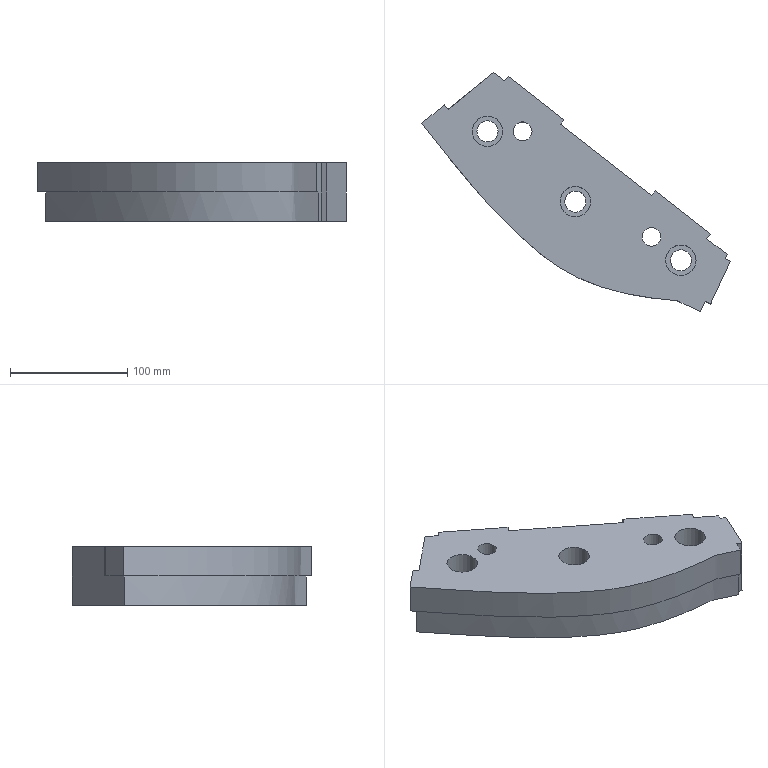Part | NX | features solid 2 | 1 solid | 34 faces | box 263.418 x 204.229 x 50 mm | volume 1065155 mm3 | plane 23 | cylinder 8 | spline 3 | commonest cylinder face diameters 18 x3 26 x3 16 x2
STEP:
#1=CARTESIAN_POINT('',(148.001,-494.484,-50.));
#2=VERTEX_POINT('',#1);
#3=CARTESIAN_POINT('',(140.001,-494.484,-50.));
#4=DIRECTION('',(0.,0.,1.));
#5=DIRECTION('',(1.,0.,0.));
#6=AXIS2_PLACEMENT_3D('',#3,#4,#5);
#7=CIRCLE('',#6,8.);
#8=EDGE_CURVE('',#2,#2,#7,.F.);
#9=ORIENTED_EDGE('',*,*,#8,.F.);
#10=EDGE_LOOP('',(#9));
#11=FACE_BOUND('',#10,.T.);
#12=CARTESIAN_POINT('',(38.001,-404.484,-50.));
#13=VERTEX_POINT('',#12);
#14=CARTESIAN_POINT('',(30.001,-404.484,-50.));
#15=DIRECTION('',(0.,0.,1.));
#16=DIRECTION('',(1.,0.,0.));
#17=AXIS2_PLACEMENT_3D('',#14,#15,#16);
#18=CIRCLE('',#17,8.);
#19=EDGE_CURVE('',#13,#13,#18,.F.);
#20=ORIENTED_EDGE('',*,*,#19,.F.);
#21=EDGE_LOOP('',(#20));
#22=FACE_BOUND('',#21,.T.);
#23=CARTESIAN_POINT('',(183.872,-553.837,-50.));
#24=VERTEX_POINT('',#23);
#25=CARTESIAN_POINT('',(-49.164,-398.414,-50.));
#26=VERTEX_POINT('',#25);
#27=CARTESIAN_POINT('',(183.872,-553.837,-50.));
#28=CARTESIAN_POINT('',(181.19,-552.587,-50.));
#29=CARTESIAN_POINT('',(177.655,-550.938,-50.));
#30=CARTESIAN_POINT('',(173.916,-549.195,-50.));
#31=CARTESIAN_POINT('',(171.6,-548.115,-50.));
#32=CARTESIAN_POINT('',(169.771,-547.262,-50.));
#33=CARTESIAN_POINT('',(168.654,-546.741,-50.));
#34=CARTESIAN_POINT('',(168.003,-546.437,-50.));
#35=CARTESIAN_POINT('',(167.64,-546.268,-50.));
#36=CARTESIAN_POINT('',(167.426,-546.168,-50.));
#37=CARTESIAN_POINT('',(167.355,-546.135,-50.));
#38=CARTESIAN_POINT('',(167.291,-546.104,-50.));
#39=CARTESIAN_POINT('',(167.361,-546.137,-50.));
#40=CARTESIAN_POINT('',(167.014,-545.975,-50.));
#41=CARTESIAN_POINT('',(166.698,-545.827,-50.));
#42=CARTESIAN_POINT('',(166.252,-545.617,-50.));
#43=CARTESIAN_POINT('',(165.74,-545.378,-50.));
#44=CARTESIAN_POINT('',(165.042,-545.046,-50.));
#45=CARTESIAN_POINT('',(164.226,-544.695,-50.));
#46=CARTESIAN_POINT('',(163.094,-544.305,-50.));
#47=CARTESIAN_POINT('',(162.195,-544.064,-50.));
#48=CARTESIAN_POINT('',(161.539,-543.93,-50.));
#49=CARTESIAN_POINT('',(161.184,-543.867,-50.));
#50=CARTESIAN_POINT('',(160.858,-543.817,-50.));
#51=CARTESIAN_POINT('',(160.755,-543.804,-50.));
#52=CARTESIAN_POINT('',(160.477,-543.771,-50.));
#53=CARTESIAN_POINT('',(160.073,-543.731,-50.));
#54=CARTESIAN_POINT('',(159.523,-543.683,-50.));
#55=CARTESIAN_POINT('',(159.037,-543.643,-50.));
#56=CARTESIAN_POINT('',(158.567,-543.607,-50.));
#57=CARTESIAN_POINT('',(158.321,-543.588,-50.));
#58=CARTESIAN_POINT('',(157.916,-543.557,-50.));
#59=CARTESIAN_POINT('',(157.244,-543.504,-50.));
#60=CARTESIAN_POINT('',(156.27,-543.425,-50.));
#61=CARTESIAN_POINT('',(155.116,-543.328,-50.));
#62=CARTESIAN_POINT('',(153.584,-543.194,-50.));
#63=CARTESIAN_POINT('',(151.666,-543.017,-50.));
#64=CARTESIAN_POINT('',(149.486,-542.802,-50.));
#65=CARTESIAN_POINT('',(146.978,-542.536,-50.));
#66=CARTESIAN_POINT('',(143.79,-542.173,-50.));
#67=CARTESIAN_POINT('',(138.237,-541.478,-50.));
#68=CARTESIAN_POINT('',(130.582,-540.33,-50.));
#69=CARTESIAN_POINT('',(123.224,-538.968,-50.));
#70=CARTESIAN_POINT('',(118.275,-537.912,-50.));
#71=CARTESIAN_POINT('',(115.449,-537.265,-50.));
#72=CARTESIAN_POINT('',(113.484,-536.797,-50.));
#73=CARTESIAN_POINT('',(111.045,-536.188,-50.));
#74=CARTESIAN_POINT('',(108.002,-535.388,-50.));
#75=CARTESIAN_POINT('',(102.684,-533.89,-50.));
#76=CARTESIAN_POINT('',(95.378,-531.535,-50.));
#77=CARTESIAN_POINT('',(88.413,-528.888,-50.));
#78=CARTESIAN_POINT('',(83.006,-526.572,-50.));
#79=CARTESIAN_POINT('',(79.163,-524.8,-50.));
#80=CARTESIAN_POINT('',(75.001,-522.73,-50.));
#81=CARTESIAN_POINT('',(71.042,-520.6,-50.));
#82=CARTESIAN_POINT('',(67.801,-518.726,-50.));
#83=CARTESIAN_POINT('',(65.566,-517.361,-50.));
#84=CARTESIAN_POINT('',(64.317,-516.578,-50.));
#85=CARTESIAN_POINT('',(63.338,-515.952,-50.));
#86=CARTESIAN_POINT('',(62.553,-515.443,-50.));
#87=CARTESIAN_POINT('',(61.419,-514.694,-50.));
#88=CARTESIAN_POINT('',(59.423,-513.345,-50.));
#89=CARTESIAN_POINT('',(56.429,-511.236,-50.));
#90=CARTESIAN_POINT('',(53.281,-508.908,-50.));
#91=CARTESIAN_POINT('',(50.978,-507.148,-50.));
#92=CARTESIAN_POINT('',(49.656,-506.124,-50.));
#93=CARTESIAN_POINT('',(48.597,-505.295,-50.));
#94=CARTESIAN_POINT('',(47.737,-504.616,-50.));
#95=CARTESIAN_POINT('',(46.527,-503.654,-50.));
#96=CARTESIAN_POINT('',(44.454,-501.988,-50.));
#97=CARTESIAN_POINT('',(41.508,-499.566,-50.));
#98=CARTESIAN_POINT('',(38.048,-496.635,-50.));
#99=CARTESIAN_POINT('',(34.6,-493.624,-50.));
#100=CARTESIAN_POINT('',(31.367,-490.714,-50.));
#101=CARTESIAN_POINT('',(28.058,-487.655,-50.));
#102=CARTESIAN_POINT('',(25.286,-485.02,-50.));
#103=CARTESIAN_POINT('',(23.09,-482.892,-50.));
#104=CARTESIAN_POINT('',(21.348,-481.181,-50.));
#105=CARTESIAN_POINT('',(19.949,-479.79,-50.));
#106=CARTESIAN_POINT('',(17.948,-477.781,-50.));
#107=CARTESIAN_POINT('',(14.47,-474.232,-50.));
#108=CARTESIAN_POINT('',(10.396,-469.946,-50.));
#109=CARTESIAN_POINT('',(6.255,-465.465,-50.));
#110=CARTESIAN_POINT('',(3.108,-461.998,-50.));
#111=CARTESIAN_POINT('',(0.4635,-459.035,-50.));
#112=CARTESIAN_POINT('',(-1.422,-456.894,-50.));
#113=CARTESIAN_POINT('',(-2.477,-455.691,-50.));
#114=CARTESIAN_POINT('',(-3.348,-454.691,-50.));
#115=CARTESIAN_POINT('',(-3.921,-454.032,-50.));
#116=CARTESIAN_POINT('',(-4.799,-453.019,-50.));
#117=CARTESIAN_POINT('',(-6.306,-451.271,-50.));
#118=CARTESIAN_POINT('',(-8.542,-448.656,-50.));
#119=CARTESIAN_POINT('',(-11.305,-445.386,-50.));
#120=CARTESIAN_POINT('',(-14.163,-441.97,-50.));
#121=CARTESIAN_POINT('',(-17.111,-438.411,-50.));
#122=CARTESIAN_POINT('',(-19.645,-435.325,-50.));
#123=CARTESIAN_POINT('',(-21.717,-432.786,-50.));
#124=CARTESIAN_POINT('',(-23.295,-430.843,-50.));
#125=CARTESIAN_POINT('',(-24.624,-429.203,-50.));
#126=CARTESIAN_POINT('',(-25.576,-428.022,-50.));
#127=CARTESIAN_POINT('',(-26.103,-427.369,-50.));
#128=CARTESIAN_POINT('',(-26.557,-426.805,-50.));
#129=CARTESIAN_POINT('',(-26.795,-426.51,-50.));
#130=CARTESIAN_POINT('',(-27.195,-426.012,-50.));
#131=CARTESIAN_POINT('',(-27.875,-425.166,-50.));
#132=CARTESIAN_POINT('',(-28.91,-423.875,-50.));
#133=CARTESIAN_POINT('',(-30.217,-422.242,-50.));
#134=CARTESIAN_POINT('',(-31.599,-420.513,-50.));
#135=CARTESIAN_POINT('',(-33.052,-418.691,-50.));
#136=CARTESIAN_POINT('',(-34.324,-417.095,-50.));
#137=CARTESIAN_POINT('',(-35.378,-415.77,-50.));
#138=CARTESIAN_POINT('',(-36.185,-414.755,-50.));
#139=CARTESIAN_POINT('',(-36.878,-413.883,-50.));
#140=CARTESIAN_POINT('',(-37.36,-413.276,-50.));
#141=CARTESIAN_POINT('',(-37.655,-412.904,-50.));
#142=CARTESIAN_POINT('',(-37.828,-412.687,-50.));
#143=CARTESIAN_POINT('',(-38.192,-412.228,-50.));
#144=CARTESIAN_POINT('',(-38.603,-411.711,-50.));
#145=CARTESIAN_POINT('',(-39.337,-410.787,-50.));
#146=CARTESIAN_POINT('',(-40.323,-409.545,-50.));
#147=CARTESIAN_POINT('',(-41.439,-408.14,-50.));
#148=CARTESIAN_POINT('',(-42.825,-406.393,-50.));
#149=CARTESIAN_POINT('',(-44.374,-404.443,-50.));
#150=CARTESIAN_POINT('',(-46.456,-401.822,-50.));
#151=CARTESIAN_POINT('',(-48.316,-399.48,-50.));
#152=CARTESIAN_POINT('',(-49.013,-398.603,-50.));
#153=CARTESIAN_POINT('',(-49.164,-398.414,-50.));
#154=B_SPLINE_CURVE_WITH_KNOTS('',3,(#27,#28,#29,#30,#31,#32,#33,#34,#35,#36,#37,#38,#39,#40,#41,#42,#43,#44,#45,#46,#47,#48,#49,#50,#51,#52,#53,#54,#55,#56,#57,#58,#59,#60,#61,#62,#63,#64,#65,#66,#67,#68,#69,#70,#71,#72,#73,#74,#75,#76,#77,#78,#79,#80,#81,#82,#83,#84,#85,#86,#87,#88,#89,#90,#91,#92,#93,#94,#95,#96,#97,#98,#99,#100,#101,#102,#103,#104,#105,#106,#107,#108,#109,#110,#111,#112,#113,#114,#115,#116,#117,#118,#119,#120,#121,#122,#123,#124,#125,#126,#127,#128,#129,#130,#131,#132,#133,#134,#135,#136,#137,#138,#139,#140,#141,#142,#143,#144,#145,#146,#147,#148,#149,#150,#151,#152,#153),.UNSPECIFIED.,.F.,.F.,(4,1,1,1,1,1,1,1,1,1,1,1,1,1,1,1,1,1,1,1,1,1,1,1,1,1,1,1,1,1,1,1,1,1,1,1,1,1,1,1,1,1,1,1,1,1,1,1,1,1,1,1,1,1,1,1,1,1,1,1,1,1,1,1,1,1,1,1,1,1,1,1,1,1,1,1,1,1,1,1,1,1,1,1,1,1,1,1,1,1,1,1,1,1,1,1,1,1,1,1,1,1,1,1,1,1,1,1,1,1,1,1,1,1,1,1,1,1,1,1,1,1,1,1,4),(0.,0.01562,0.02344,0.03125,0.03906,0.04688,0.05078,0.05469,0.05859,0.06055,0.06152,0.0625,0.06348,0.06445,0.06641,0.06836,0.07031,0.07422,0.07812,0.08203,0.08398,0.08496,0.08594,0.08691,0.08789,0.08984,0.0918,0.09277,0.09375,0.09473,0.0957,0.09766,0.1016,0.1055,0.1094,0.1172,0.125,0.1328,0.1406,0.1562,0.1875,0.2188,0.2344,0.2422,0.25,0.2578,0.2656,0.2812,0.3125,0.3438,0.3594,0.375,0.3906,0.4062,0.4219,0.4297,0.4336,0.4375,0.4414,0.4453,0.4531,0.4688,0.4844,0.4922,0.4961,0.5,0.5039,0.5078,0.5156,0.5312,0.5469,0.5625,0.5781,0.5938,0.6094,0.6172,0.625,0.6328,0.6406,0.6562,0.6875,0.7031,0.7188,0.7344,0.7422,0.7461,0.75,0.7539,0.7578,0.7656,0.7812,0.7969,0.8125,0.8281,0.8438,0.8516,0.8594,0.8672,0.8711,0.873,0.875,0.877,0.8789,0.8828,0.8906,0.8984,0.9062,0.9141,0.9219,0.9258,0.9297,0.9336,0.9355,0.9365,0.9375,0.9385,0.9395,0.9414,0.9453,0.9492,0.9531,0.9609,0.9688,0.9844,1.),.UNSPECIFIED.);
#155=EDGE_CURVE('',#24,#26,#154,.T.);
#156=ORIENTED_EDGE('',*,*,#155,.T.);
#157=CARTESIAN_POINT('',(5.511,-354.14,-50.));
#158=VERTEX_POINT('',#157);
#159=CARTESIAN_POINT('',(-49.136,-398.392,-50.));
#160=DIRECTION('',(0.7771,0.6293,0.));
#161=VECTOR('',#160,1000.);
#162=LINE('',#159,#161);
#163=EDGE_CURVE('',#26,#158,#162,.T.);
#164=ORIENTED_EDGE('',*,*,#163,.T.);
#165=CARTESIAN_POINT('',(14.909,-361.482,-50.));
#166=VERTEX_POINT('',#165);
#167=CARTESIAN_POINT('',(87.506,-418.202,-50.));
#168=DIRECTION('',(0.788,-0.6157,0.));
#169=VECTOR('',#168,1000.);
#170=LINE('',#167,#169);
#171=EDGE_CURVE('',#158,#166,#170,.T.);
#172=ORIENTED_EDGE('',*,*,#171,.T.);
#173=CARTESIAN_POINT('',(17.987,-357.542,-50.));
#174=VERTEX_POINT('',#173);
#175=CARTESIAN_POINT('',(17.987,-357.542,-50.));
#176=DIRECTION('',(0.6157,0.788,0.));
#177=VECTOR('',#176,1000.);
#178=LINE('',#175,#177);
#179=EDGE_CURVE('',#166,#174,#178,.T.);
#180=ORIENTED_EDGE('',*,*,#179,.T.);
#181=CARTESIAN_POINT('',(65.268,-394.482,-50.));
#182=VERTEX_POINT('',#181);
#183=CARTESIAN_POINT('',(90.585,-414.262,-50.));
#184=DIRECTION('',(0.788,-0.6157,0.));
#185=VECTOR('',#184,1000.);
#186=LINE('',#183,#185);
#187=EDGE_CURVE('',#174,#182,#186,.T.);
#188=ORIENTED_EDGE('',*,*,#187,.T.);
#189=CARTESIAN_POINT('',(62.189,-398.422,-50.));
#190=VERTEX_POINT('',#189);
#191=CARTESIAN_POINT('',(65.268,-394.482,-50.));
#192=DIRECTION('',(0.6157,0.788,0.));
#193=VECTOR('',#192,1000.);
#194=LINE('',#191,#193);
#195=EDGE_CURVE('',#190,#182,#194,.T.);
#196=ORIENTED_EDGE('',*,*,#195,.F.);
#197=CARTESIAN_POINT('',(139.939,-459.167,-50.));
#198=VERTEX_POINT('',#197);
#199=CARTESIAN_POINT('',(87.506,-418.202,-50.));
#200=DIRECTION('',(0.788,-0.6157,0.));
#201=VECTOR('',#200,1000.);
#202=LINE('',#199,#201);
#203=EDGE_CURVE('',#190,#198,#202,.T.);
#204=ORIENTED_EDGE('',*,*,#203,.T.);
#205=CARTESIAN_POINT('',(143.017,-455.226,-50.));
#206=VERTEX_POINT('',#205);
#207=CARTESIAN_POINT('',(143.017,-455.226,-50.));
#208=DIRECTION('',(0.6157,0.788,0.));
#209=VECTOR('',#208,1000.);
#210=LINE('',#207,#209);
#211=EDGE_CURVE('',#198,#206,#210,.T.);
#212=ORIENTED_EDGE('',*,*,#211,.T.);
#213=CARTESIAN_POINT('',(190.298,-492.166,-50.));
#214=VERTEX_POINT('',#213);
#215=CARTESIAN_POINT('',(90.585,-414.262,-50.));
#216=DIRECTION('',(0.788,-0.6157,0.));
#217=VECTOR('',#216,1000.);
#218=LINE('',#215,#217);
#219=EDGE_CURVE('',#206,#214,#218,.T.);
#220=ORIENTED_EDGE('',*,*,#219,.T.);
#221=CARTESIAN_POINT('',(187.22,-496.106,-50.));
#222=VERTEX_POINT('',#221);
#223=CARTESIAN_POINT('',(190.298,-492.166,-50.));
#224=DIRECTION('',(0.6157,0.788,0.));
#225=VECTOR('',#224,1000.);
#226=LINE('',#223,#225);
#227=EDGE_CURVE('',#222,#214,#226,.T.);
#228=ORIENTED_EDGE('',*,*,#227,.F.);
#229=CARTESIAN_POINT('',(204.497,-509.605,-50.));
#230=VERTEX_POINT('',#229);
#231=CARTESIAN_POINT('',(87.506,-418.202,-50.));
#232=DIRECTION('',(0.788,-0.6157,0.));
#233=VECTOR('',#232,1000.);
#234=LINE('',#231,#233);
#235=EDGE_CURVE('',#222,#230,#234,.T.);
#236=ORIENTED_EDGE('',*,*,#235,.T.);
#237=CARTESIAN_POINT('',(202.718,-513.422,-50.));
#238=VERTEX_POINT('',#237);
#239=CARTESIAN_POINT('',(-189.498,-1354.531,-50.));
#240=DIRECTION('',(0.4226,0.9063,0.));
#241=VECTOR('',#240,1000.);
#242=LINE('',#239,#241);
#243=EDGE_CURVE('',#238,#230,#242,.T.);
#244=ORIENTED_EDGE('',*,*,#243,.F.);
#245=CARTESIAN_POINT('',(207.249,-515.535,-50.));
#246=VERTEX_POINT('',#245);
#247=CARTESIAN_POINT('',(-130.442,-358.067,-50.));
#248=DIRECTION('',(0.9063,-0.4226,0.));
#249=VECTOR('',#248,1000.);
#250=LINE('',#247,#249);
#251=EDGE_CURVE('',#238,#246,#250,.T.);
#252=ORIENTED_EDGE('',*,*,#251,.T.);
#253=CARTESIAN_POINT('',(190.345,-551.787,-50.));
#254=VERTEX_POINT('',#253);
#255=CARTESIAN_POINT('',(196.684,-538.192,-50.));
#256=DIRECTION('',(-0.4226,-0.9063,0.));
#257=VECTOR('',#256,1000.);
#258=LINE('',#255,#257);
#259=EDGE_CURVE('',#254,#246,#258,.F.);
#260=ORIENTED_EDGE('',*,*,#259,.F.);
#261=CARTESIAN_POINT('',(185.813,-549.674,-50.));
#262=VERTEX_POINT('',#261);
#263=CARTESIAN_POINT('',(185.813,-549.674,-50.));
#264=DIRECTION('',(0.9063,-0.4226,0.));
#265=VECTOR('',#264,1000.);
#266=LINE('',#263,#265);
#267=EDGE_CURVE('',#262,#254,#266,.T.);
#268=ORIENTED_EDGE('',*,*,#267,.F.);
#269=CARTESIAN_POINT('',(-189.498,-1354.531,-50.));
#270=DIRECTION('',(0.4226,0.9063,0.));
#271=VECTOR('',#270,1000.);
#272=LINE('',#269,#271);
#273=EDGE_CURVE('',#24,#262,#272,.T.);
#274=ORIENTED_EDGE('',*,*,#273,.F.);
#275=EDGE_LOOP('',(#156,#164,#172,#180,#188,#196,#204,#212,#220,#228,#236,#244,#252,#260,#268,#274));
#276=FACE_BOUND('',#275,.T.);
#277=CARTESIAN_POINT('',(9.001,-404.484,-50.));
#278=VERTEX_POINT('',#277);
#279=CARTESIAN_POINT('',(0.001372,-404.484,-50.));
#280=DIRECTION('',(0.,0.,1.));
#281=DIRECTION('',(1.,0.,0.));
#282=AXIS2_PLACEMENT_3D('',#279,#280,#281);
#283=CIRCLE('',#282,9.);
#284=EDGE_CURVE('',#278,#278,#283,.F.);
#285=ORIENTED_EDGE('',*,*,#284,.F.);
#286=EDGE_LOOP('',(#285));
#287=FACE_BOUND('',#286,.T.);
#288=CARTESIAN_POINT('',(84.001,-464.484,-50.));
#289=VERTEX_POINT('',#288);
#290=CARTESIAN_POINT('',(75.001,-464.484,-50.));
#291=DIRECTION('',(0.,0.,1.));
#292=DIRECTION('',(1.,0.,0.));
#293=AXIS2_PLACEMENT_3D('',#290,#291,#292);
#294=CIRCLE('',#293,9.);
#295=EDGE_CURVE('',#289,#289,#294,.F.);
#296=ORIENTED_EDGE('',*,*,#295,.F.);
#297=EDGE_LOOP('',(#296));
#298=FACE_BOUND('',#297,.T.);
#299=CARTESIAN_POINT('',(174.001,-514.484,-50.));
#300=VERTEX_POINT('',#299);
#301=CARTESIAN_POINT('',(165.001,-514.484,-50.));
#302=DIRECTION('',(0.,0.,1.));
#303=DIRECTION('',(1.,0.,0.));
#304=AXIS2_PLACEMENT_3D('',#301,#302,#303);
#305=CIRCLE('',#304,9.);
#306=EDGE_CURVE('',#300,#300,#305,.F.);
#307=ORIENTED_EDGE('',*,*,#306,.F.);
#308=EDGE_LOOP('',(#307));
#309=FACE_BOUND('',#308,.T.);
#310=CARTESIAN_POINT('',(-522.658,-1199.176,-50.));
#311=DIRECTION('',(0.,0.,1.));
#312=DIRECTION('',(1.,0.,0.));
#313=AXIS2_PLACEMENT_3D('',#310,#311,#312);
#314=PLANE('',#313);
#315=ADVANCED_FACE('',(#11,#22,#276,#287,#298,#309),#314,.F.);
#316=CARTESIAN_POINT('',(204.497,-509.605,0.));
#317=VERTEX_POINT('',#316);
#318=CARTESIAN_POINT('',(202.718,-513.422,0.));
#319=VERTEX_POINT('',#318);
#320=CARTESIAN_POINT('',(-641.983,-2324.887,0.));
#321=DIRECTION('',(-0.4226,-0.9063,0.));
#322=VECTOR('',#321,1000.);
#323=LINE('',#320,#322);
#324=EDGE_CURVE('',#317,#319,#323,.T.);
#325=ORIENTED_EDGE('',*,*,#324,.T.);
#326=CARTESIAN_POINT('',(202.718,-513.422,-70.));
#327=DIRECTION('',(0.,0.,-1.));
#328=VECTOR('',#327,1000.);
#329=LINE('',#326,#328);
#330=EDGE_CURVE('',#319,#238,#329,.T.);
#331=ORIENTED_EDGE('',*,*,#330,.T.);
#332=ORIENTED_EDGE('',*,*,#243,.T.);
#333=CARTESIAN_POINT('',(204.497,-509.605,-70.));
#334=DIRECTION('',(0.,0.,1.));
#335=VECTOR('',#334,1000.);
#336=LINE('',#333,#335);
#337=EDGE_CURVE('',#230,#317,#336,.T.);
#338=ORIENTED_EDGE('',*,*,#337,.T.);
#339=EDGE_LOOP('',(#325,#331,#332,#338));
#340=FACE_BOUND('',#339,.T.);
#341=CARTESIAN_POINT('',(-641.983,-2324.887,-70.));
#342=DIRECTION('',(0.9063,-0.4226,0.));
#343=DIRECTION('',(0.4226,0.9063,0.));
#344=AXIS2_PLACEMENT_3D('',#341,#342,#343);
#345=PLANE('',#344);
#346=ADVANCED_FACE('',(#340),#345,.T.);
#347=CARTESIAN_POINT('',(14.909,-361.482,0.));
#348=VERTEX_POINT('',#347);
#349=CARTESIAN_POINT('',(14.909,-361.482,-25.));
#350=DIRECTION('',(0.,0.,-1.));
#351=VECTOR('',#350,1000.);
#352=LINE('',#349,#351);
#353=EDGE_CURVE('',#348,#166,#352,.T.);
#354=ORIENTED_EDGE('',*,*,#353,.T.);
#355=ORIENTED_EDGE('',*,*,#171,.F.);
#356=CARTESIAN_POINT('',(5.511,-354.14,0.));
#357=VERTEX_POINT('',#356);
#358=CARTESIAN_POINT('',(5.511,-354.14,-70.));
#359=DIRECTION('',(0.,0.,-1.));
#360=VECTOR('',#359,1000.);
#361=LINE('',#358,#360);
#362=EDGE_CURVE('',#357,#158,#361,.T.);
#363=ORIENTED_EDGE('',*,*,#362,.F.);
#364=CARTESIAN_POINT('',(-73.655,-292.288,0.));
#365=DIRECTION('',(-0.788,0.6157,0.));
#366=VECTOR('',#365,1000.);
#367=LINE('',#364,#366);
#368=EDGE_CURVE('',#348,#357,#367,.T.);
#369=ORIENTED_EDGE('',*,*,#368,.F.);
#370=EDGE_LOOP('',(#354,#355,#363,#369));
#371=FACE_BOUND('',#370,.T.);
#372=CARTESIAN_POINT('',(-73.655,-292.288,-70.));
#373=DIRECTION('',(-0.6157,-0.788,0.));
#374=DIRECTION('',(0.788,-0.6157,0.));
#375=AXIS2_PLACEMENT_3D('',#372,#373,#374);
#376=PLANE('',#375);
#377=ADVANCED_FACE('',(#371),#376,.F.);
#378=ORIENTED_EDGE('',*,*,#203,.F.);
#379=CARTESIAN_POINT('',(62.189,-398.422,0.));
#380=VERTEX_POINT('',#379);
#381=CARTESIAN_POINT('',(62.189,-398.422,-25.));
#382=DIRECTION('',(0.,0.,-1.));
#383=VECTOR('',#382,1000.);
#384=LINE('',#381,#383);
#385=EDGE_CURVE('',#380,#190,#384,.T.);
#386=ORIENTED_EDGE('',*,*,#385,.F.);
#387=CARTESIAN_POINT('',(139.939,-459.167,0.));
#388=VERTEX_POINT('',#387);
#389=CARTESIAN_POINT('',(-73.655,-292.288,0.));
#390=DIRECTION('',(-0.788,0.6157,0.));
#391=VECTOR('',#390,1000.);
#392=LINE('',#389,#391);
#393=EDGE_CURVE('',#388,#380,#392,.T.);
#394=ORIENTED_EDGE('',*,*,#393,.F.);
#395=CARTESIAN_POINT('',(139.939,-459.167,-25.));
#396=DIRECTION('',(0.,0.,-1.));
#397=VECTOR('',#396,1000.);
#398=LINE('',#395,#397);
#399=EDGE_CURVE('',#388,#198,#398,.T.);
#400=ORIENTED_EDGE('',*,*,#399,.T.);
#401=EDGE_LOOP('',(#378,#386,#394,#400));
#402=FACE_BOUND('',#401,.T.);
#403=CARTESIAN_POINT('',(-73.655,-292.288,-70.));
#404=DIRECTION('',(-0.6157,-0.788,0.));
#405=DIRECTION('',(0.788,-0.6157,0.));
#406=AXIS2_PLACEMENT_3D('',#403,#404,#405);
#407=PLANE('',#406);
#408=ADVANCED_FACE('',(#402),#407,.F.);
#409=ORIENTED_EDGE('',*,*,#235,.F.);
#410=CARTESIAN_POINT('',(187.22,-496.106,0.));
#411=VERTEX_POINT('',#410);
#412=CARTESIAN_POINT('',(187.22,-496.106,-25.));
#413=DIRECTION('',(0.,0.,-1.));
#414=VECTOR('',#413,1000.);
#415=LINE('',#412,#414);
#416=EDGE_CURVE('',#411,#222,#415,.T.);
#417=ORIENTED_EDGE('',*,*,#416,.F.);
#418=CARTESIAN_POINT('',(-73.655,-292.288,0.));
#419=DIRECTION('',(-0.788,0.6157,0.));
#420=VECTOR('',#419,1000.);
#421=LINE('',#418,#420);
#422=EDGE_CURVE('',#317,#411,#421,.T.);
#423=ORIENTED_EDGE('',*,*,#422,.F.);
#424=ORIENTED_EDGE('',*,*,#337,.F.);
#425=EDGE_LOOP('',(#409,#417,#423,#424));
#426=FACE_BOUND('',#425,.T.);
#427=CARTESIAN_POINT('',(-73.655,-292.288,-70.));
#428=DIRECTION('',(-0.6157,-0.788,0.));
#429=DIRECTION('',(0.788,-0.6157,0.));
#430=AXIS2_PLACEMENT_3D('',#427,#428,#429);
#431=PLANE('',#430);
#432=ADVANCED_FACE('',(#426),#431,.F.);
#433=CARTESIAN_POINT('',(-36.74,-381.92,0.));
#434=VERTEX_POINT('',#433);
#435=CARTESIAN_POINT('',(-36.645,-382.038,0.));
#436=VERTEX_POINT('',#435);
#437=CARTESIAN_POINT('',(172.333,-643.328,0.));
#438=DIRECTION('',(0.6246,-0.7809,0.));
#439=VECTOR('',#438,1000.);
#440=LINE('',#437,#439);
#441=EDGE_CURVE('',#434,#436,#440,.T.);
#442=ORIENTED_EDGE('',*,*,#441,.F.);
#443=CARTESIAN_POINT('',(-56.169,-397.653,0.));
#444=VERTEX_POINT('',#443);
#445=CARTESIAN_POINT('',(-729.911,-943.239,0.));
#446=DIRECTION('',(0.7771,0.6293,0.));
#447=VECTOR('',#446,1000.);
#448=LINE('',#445,#447);
#449=EDGE_CURVE('',#444,#434,#448,.T.);
#450=ORIENTED_EDGE('',*,*,#449,.F.);
#451=CARTESIAN_POINT('',(181.759,-558.369,0.));
#452=VERTEX_POINT('',#451);
#453=CARTESIAN_POINT('',(181.759,-558.369,0.));
#454=CARTESIAN_POINT('',(180.377,-557.725,0.));
#455=CARTESIAN_POINT('',(177.614,-556.435,0.));
#456=CARTESIAN_POINT('',(173.468,-554.507,0.));
#457=CARTESIAN_POINT('',(169.33,-552.558,0.));
#458=CARTESIAN_POINT('',(165.16,-550.686,0.));
#459=CARTESIAN_POINT('',(161.789,-548.882,0.));
#460=CARTESIAN_POINT('',(158.584,-548.621,0.));
#461=CARTESIAN_POINT('',(155.372,-548.376,0.));
#462=CARTESIAN_POINT('',(151.378,-548.02,0.));
#463=CARTESIAN_POINT('',(145.022,-547.373,0.));
#464=CARTESIAN_POINT('',(137.148,-546.396,0.));
#465=CARTESIAN_POINT('',(124.716,-544.448,0.));
#466=CARTESIAN_POINT('',(109.513,-541.229,0.));
#467=CARTESIAN_POINT('',(91.916,-535.869,0.));
#468=CARTESIAN_POINT('',(75.07,-528.749,0.));
#469=CARTESIAN_POINT('',(59.108,-519.629,0.));
#470=CARTESIAN_POINT('',(44.023,-508.274,0.));
#471=CARTESIAN_POINT('',(29.606,-496.111,0.));
#472=CARTESIAN_POINT('',(11.575,-478.894,0.));
#473=CARTESIAN_POINT('',(-9.357,-455.901,0.));
#474=CARTESIAN_POINT('',(-32.981,-426.975,0.));
#475=CARTESIAN_POINT('',(-48.389,-407.381,0.));
#476=CARTESIAN_POINT('',(-56.169,-397.653,0.));
#477=B_SPLINE_CURVE_WITH_KNOTS('',3,(#453,#454,#455,#456,#457,#458,#459,#460,#461,#462,#463,#464,#465,#466,#467,#468,#469,#470,#471,#472,#473,#474,#475,#476),.UNSPECIFIED.,.F.,.F.,(4,1,1,1,1,1,1,1,1,1,1,1,1,1,1,1,1,1,1,1,1,4),(0.7207,0.7253,0.7298,0.7344,0.739,0.7435,0.7458,0.7481,0.7527,0.7573,0.7664,0.7756,0.7938,0.8121,0.8304,0.8487,0.867,0.8853,0.9036,0.9402,0.9768,1.013),.UNSPECIFIED.);
#478=EDGE_CURVE('',#452,#444,#477,.T.);
#479=ORIENTED_EDGE('',*,*,#478,.F.);
#480=CARTESIAN_POINT('',(185.813,-549.674,0.));
#481=VERTEX_POINT('',#480);
#482=CARTESIAN_POINT('',(-189.498,-1354.531,0.));
#483=DIRECTION('',(0.4226,0.9063,0.));
#484=VECTOR('',#483,1000.);
#485=LINE('',#482,#484);
#486=EDGE_CURVE('',#452,#481,#485,.T.);
#487=ORIENTED_EDGE('',*,*,#486,.T.);
#488=CARTESIAN_POINT('',(190.345,-551.787,0.));
#489=VERTEX_POINT('',#488);
#490=CARTESIAN_POINT('',(185.813,-549.674,0.));
#491=DIRECTION('',(0.9063,-0.4226,0.));
#492=VECTOR('',#491,1000.);
#493=LINE('',#490,#492);
#494=EDGE_CURVE('',#481,#489,#493,.T.);
#495=ORIENTED_EDGE('',*,*,#494,.T.);
#496=CARTESIAN_POINT('',(207.249,-515.535,0.));
#497=VERTEX_POINT('',#496);
#498=CARTESIAN_POINT('',(186.29,-560.482,0.));
#499=DIRECTION('',(0.4226,0.9063,0.));
#500=VECTOR('',#499,1000.);
#501=LINE('',#498,#500);
#502=EDGE_CURVE('',#489,#497,#501,.T.);
#503=ORIENTED_EDGE('',*,*,#502,.T.);
#504=CARTESIAN_POINT('',(-130.442,-358.067,0.));
#505=DIRECTION('',(0.9063,-0.4226,0.));
#506=VECTOR('',#505,1000.);
#507=LINE('',#504,#506);
#508=EDGE_CURVE('',#319,#497,#507,.T.);
#509=ORIENTED_EDGE('',*,*,#508,.F.);
#510=ORIENTED_EDGE('',*,*,#324,.F.);
#511=ORIENTED_EDGE('',*,*,#422,.T.);
#512=CARTESIAN_POINT('',(190.298,-492.166,0.));
#513=VERTEX_POINT('',#512);
#514=CARTESIAN_POINT('',(154.943,-537.418,0.));
#515=DIRECTION('',(0.6157,0.788,0.));
#516=VECTOR('',#515,1000.);
#517=LINE('',#514,#516);
#518=EDGE_CURVE('',#411,#513,#517,.T.);
#519=ORIENTED_EDGE('',*,*,#518,.T.);
#520=CARTESIAN_POINT('',(143.017,-455.226,0.));
#521=VERTEX_POINT('',#520);
#522=CARTESIAN_POINT('',(90.585,-414.262,0.));
#523=DIRECTION('',(0.788,-0.6157,0.));
#524=VECTOR('',#523,1000.);
#525=LINE('',#522,#524);
#526=EDGE_CURVE('',#521,#513,#525,.T.);
#527=ORIENTED_EDGE('',*,*,#526,.F.);
#528=CARTESIAN_POINT('',(107.662,-500.479,0.));
#529=DIRECTION('',(0.6157,0.788,0.));
#530=VECTOR('',#529,1000.);
#531=LINE('',#528,#530);
#532=EDGE_CURVE('',#388,#521,#531,.T.);
#533=ORIENTED_EDGE('',*,*,#532,.F.);
#534=ORIENTED_EDGE('',*,*,#393,.T.);
#535=CARTESIAN_POINT('',(65.268,-394.482,0.));
#536=VERTEX_POINT('',#535);
#537=CARTESIAN_POINT('',(29.913,-439.734,0.));
#538=DIRECTION('',(0.6157,0.788,0.));
#539=VECTOR('',#538,1000.);
#540=LINE('',#537,#539);
#541=EDGE_CURVE('',#380,#536,#540,.T.);
#542=ORIENTED_EDGE('',*,*,#541,.T.);
#543=CARTESIAN_POINT('',(17.987,-357.542,0.));
#544=VERTEX_POINT('',#543);
#545=CARTESIAN_POINT('',(90.585,-414.262,0.));
#546=DIRECTION('',(0.788,-0.6157,0.));
#547=VECTOR('',#546,1000.);
#548=LINE('',#545,#547);
#549=EDGE_CURVE('',#544,#536,#548,.T.);
#550=ORIENTED_EDGE('',*,*,#549,.F.);
#551=CARTESIAN_POINT('',(-17.368,-402.794,0.));
#552=DIRECTION('',(0.6157,0.788,0.));
#553=VECTOR('',#552,1000.);
#554=LINE('',#551,#553);
#555=EDGE_CURVE('',#348,#544,#554,.T.);
#556=ORIENTED_EDGE('',*,*,#555,.F.);
#557=ORIENTED_EDGE('',*,*,#368,.T.);
#558=CARTESIAN_POINT('',(-33.62,-385.828,0.));
#559=VERTEX_POINT('',#558);
#560=CARTESIAN_POINT('',(-49.136,-398.392,0.));
#561=DIRECTION('',(0.7771,0.6293,0.));
#562=VECTOR('',#561,1000.);
#563=LINE('',#560,#562);
#564=EDGE_CURVE('',#559,#357,#563,.T.);
#565=ORIENTED_EDGE('',*,*,#564,.F.);
#566=CARTESIAN_POINT('',(-33.62,-385.828,0.));
#567=CARTESIAN_POINT('',(-34.628,-384.563,0.));
#568=CARTESIAN_POINT('',(-35.636,-383.3,0.));
#569=CARTESIAN_POINT('',(-36.645,-382.038,0.));
#570=B_SPLINE_CURVE_WITH_KNOTS('',3,(#566,#567,#568,#569),.UNSPECIFIED.,.F.,.F.,(4,4),(0.2673,0.2722),.UNSPECIFIED.);
#571=EDGE_CURVE('',#559,#436,#570,.T.);
#572=ORIENTED_EDGE('',*,*,#571,.T.);
#573=EDGE_LOOP('',(#442,#450,#479,#487,#495,#503,#509,#510,#511,#519,#527,#533,#534,#542,#550,#556,#557,#565,#572));
#574=FACE_BOUND('',#573,.T.);
#575=CARTESIAN_POINT('',(88.001,-464.484,0.));
#576=VERTEX_POINT('',#575);
#577=CARTESIAN_POINT('',(75.001,-464.484,0.));
#578=DIRECTION('',(0.,0.,1.));
#579=DIRECTION('',(1.,0.,0.));
#580=AXIS2_PLACEMENT_3D('',#577,#578,#579);
#581=CIRCLE('',#580,13.);
#582=EDGE_CURVE('',#576,#576,#581,.F.);
#583=ORIENTED_EDGE('',*,*,#582,.T.);
#584=EDGE_LOOP('',(#583));
#585=FACE_BOUND('',#584,.T.);
#586=CARTESIAN_POINT('',(38.001,-404.484,0.));
#587=VERTEX_POINT('',#586);
#588=CARTESIAN_POINT('',(30.001,-404.484,0.));
#589=DIRECTION('',(0.,0.,1.));
#590=DIRECTION('',(1.,0.,0.));
#591=AXIS2_PLACEMENT_3D('',#588,#589,#590);
#592=CIRCLE('',#591,8.);
#593=EDGE_CURVE('',#587,#587,#592,.F.);
#594=ORIENTED_EDGE('',*,*,#593,.T.);
#595=EDGE_LOOP('',(#594));
#596=FACE_BOUND('',#595,.T.);
#597=CARTESIAN_POINT('',(148.001,-494.484,0.));
#598=VERTEX_POINT('',#597);
#599=CARTESIAN_POINT('',(140.001,-494.484,0.));
#600=DIRECTION('',(0.,0.,1.));
#601=DIRECTION('',(1.,0.,0.));
#602=AXIS2_PLACEMENT_3D('',#599,#600,#601);
#603=CIRCLE('',#602,8.);
#604=EDGE_CURVE('',#598,#598,#603,.F.);
#605=ORIENTED_EDGE('',*,*,#604,.T.);
#606=EDGE_LOOP('',(#605));
#607=FACE_BOUND('',#606,.T.);
#608=CARTESIAN_POINT('',(13.001,-404.484,0.));
#609=VERTEX_POINT('',#608);
#610=CARTESIAN_POINT('',(0.001372,-404.484,0.));
#611=DIRECTION('',(0.,0.,1.));
#612=DIRECTION('',(1.,0.,0.));
#613=AXIS2_PLACEMENT_3D('',#610,#611,#612);
#614=CIRCLE('',#613,13.);
#615=EDGE_CURVE('',#609,#609,#614,.F.);
#616=ORIENTED_EDGE('',*,*,#615,.T.);
#617=EDGE_LOOP('',(#616));
#618=FACE_BOUND('',#617,.T.);
#619=CARTESIAN_POINT('',(178.001,-514.484,0.));
#620=VERTEX_POINT('',#619);
#621=CARTESIAN_POINT('',(165.001,-514.484,0.));
#622=DIRECTION('',(0.,0.,1.));
#623=DIRECTION('',(1.,0.,0.));
#624=AXIS2_PLACEMENT_3D('',#621,#622,#623);
#625=CIRCLE('',#624,13.);
#626=EDGE_CURVE('',#620,#620,#625,.F.);
#627=ORIENTED_EDGE('',*,*,#626,.T.);
#628=EDGE_LOOP('',(#627));
#629=FACE_BOUND('',#628,.T.);
#630=CARTESIAN_POINT('',(-522.658,-1199.176,0.));
#631=DIRECTION('',(0.,0.,1.));
#632=DIRECTION('',(1.,0.,0.));
#633=AXIS2_PLACEMENT_3D('',#630,#631,#632);
#634=PLANE('',#633);
#635=ADVANCED_FACE('',(#574,#585,#596,#607,#618,#629),#634,.T.);
#636=CARTESIAN_POINT('',(-36.74,-381.92,-25.));
#637=VERTEX_POINT('',#636);
#638=CARTESIAN_POINT('',(-36.645,-382.038,-25.));
#639=VERTEX_POINT('',#638);
#640=CARTESIAN_POINT('',(-99.105,-303.943,-25.));
#641=DIRECTION('',(0.6246,-0.7809,0.));
#642=VECTOR('',#641,1000.);
#643=LINE('',#640,#642);
#644=EDGE_CURVE('',#637,#639,#643,.T.);
#645=ORIENTED_EDGE('',*,*,#644,.T.);
#646=CARTESIAN_POINT('',(-33.62,-385.828,-25.));
#647=VERTEX_POINT('',#646);
#648=CARTESIAN_POINT('',(-33.62,-385.828,-25.));
#649=CARTESIAN_POINT('',(-34.626,-384.565,-25.));
#650=CARTESIAN_POINT('',(-35.634,-383.302,-25.));
#651=CARTESIAN_POINT('',(-36.645,-382.038,-25.));
#652=B_SPLINE_CURVE_WITH_KNOTS('',3,(#648,#649,#650,#651),.UNSPECIFIED.,.F.,.F.,(4,4),(0.9839,1.),.UNSPECIFIED.);
#653=EDGE_CURVE('',#647,#639,#652,.T.);
#654=ORIENTED_EDGE('',*,*,#653,.F.);
#655=CARTESIAN_POINT('',(-49.164,-398.414,-25.));
#656=VERTEX_POINT('',#655);
#657=CARTESIAN_POINT('',(12.074,-348.825,-25.));
#658=DIRECTION('',(0.7771,0.6293,0.));
#659=VECTOR('',#658,1000.);
#660=LINE('',#657,#659);
#661=EDGE_CURVE('',#656,#647,#660,.T.);
#662=ORIENTED_EDGE('',*,*,#661,.F.);
#663=CARTESIAN_POINT('',(183.872,-553.837,-25.));
#664=VERTEX_POINT('',#663);
#665=CARTESIAN_POINT('',(-49.164,-398.414,-25.));
#666=CARTESIAN_POINT('',(-41.611,-407.894,-25.));
#667=CARTESIAN_POINT('',(-26.612,-426.946,-25.));
#668=CARTESIAN_POINT('',(-3.522,-455.002,-25.));
#669=CARTESIAN_POINT('',(16.93,-477.218,-25.));
#670=CARTESIAN_POINT('',(34.527,-493.789,-25.));
#671=CARTESIAN_POINT('',(48.552,-505.48,-25.));
#672=CARTESIAN_POINT('',(63.216,-516.344,-25.));
#673=CARTESIAN_POINT('',(78.961,-525.076,-25.));
#674=CARTESIAN_POINT('',(95.741,-531.923,-25.));
#675=CARTESIAN_POINT('',(113.385,-537.036,-25.));
#676=CARTESIAN_POINT('',(128.276,-540.004,-25.));
#677=CARTESIAN_POINT('',(138.824,-541.557,-25.));
#678=CARTESIAN_POINT('',(144.878,-542.306,-25.));
#679=CARTESIAN_POINT('',(149.437,-542.805,-25.));
#680=CARTESIAN_POINT('',(154.015,-543.238,-25.));
#681=CARTESIAN_POINT('',(157.84,-543.566,-25.));
#682=CARTESIAN_POINT('',(160.918,-543.766,-25.));
#683=CARTESIAN_POINT('',(163.86,-544.433,-25.));
#684=CARTESIAN_POINT('',(167.289,-546.128,-25.));
#685=CARTESIAN_POINT('',(171.441,-548.035,-25.));
#686=CARTESIAN_POINT('',(176.964,-550.62,-25.));
#687=CARTESIAN_POINT('',(181.109,-552.549,-25.));
#688=CARTESIAN_POINT('',(183.872,-553.837,-25.));
#689=B_SPLINE_CURVE_WITH_KNOTS('',3,(#665,#666,#667,#668,#669,#670,#671,#672,#673,#674,#675,#676,#677,#678,#679,#680,#681,#682,#683,#684,#685,#686,#687,#688),.UNSPECIFIED.,.F.,.F.,(4,1,1,1,1,1,1,1,1,1,1,1,1,1,1,1,1,1,1,1,1,4),(1.214,1.25,1.286,1.323,1.341,1.359,1.377,1.396,1.414,1.432,1.45,1.459,1.464,1.468,1.473,1.477,1.48,1.482,1.486,1.491,1.496,1.505),.UNSPECIFIED.);
#690=EDGE_CURVE('',#664,#656,#689,.F.);
#691=ORIENTED_EDGE('',*,*,#690,.F.);
#692=CARTESIAN_POINT('',(181.759,-558.369,-25.));
#693=VERTEX_POINT('',#692);
#694=CARTESIAN_POINT('',(181.759,-558.369,-25.));
#695=DIRECTION('',(-0.4226,-0.9063,0.));
#696=VECTOR('',#695,1000.);
#697=LINE('',#694,#696);
#698=EDGE_CURVE('',#664,#693,#697,.T.);
#699=ORIENTED_EDGE('',*,*,#698,.T.);
#700=CARTESIAN_POINT('',(-56.169,-397.653,-25.));
#701=VERTEX_POINT('',#700);
#702=CARTESIAN_POINT('',(181.759,-558.369,-25.));
#703=CARTESIAN_POINT('',(180.364,-557.718,-25.));
#704=CARTESIAN_POINT('',(177.574,-556.417,-25.));
#705=CARTESIAN_POINT('',(173.388,-554.469,-25.));
#706=CARTESIAN_POINT('',(169.208,-552.504,-25.));
#707=CARTESIAN_POINT('',(165.002,-550.602,-25.));
#708=CARTESIAN_POINT('',(161.582,-548.817,-25.));
#709=CARTESIAN_POINT('',(158.329,-548.611,-25.));
#710=CARTESIAN_POINT('',(155.101,-548.347,-25.));
#711=CARTESIAN_POINT('',(151.076,-547.993,-25.));
#712=CARTESIAN_POINT('',(144.675,-547.332,-25.));
#713=CARTESIAN_POINT('',(136.744,-546.341,-25.));
#714=CARTESIAN_POINT('',(124.222,-544.358,-25.));
#715=CARTESIAN_POINT('',(108.908,-541.079,-25.));
#716=CARTESIAN_POINT('',(91.182,-535.61,-25.));
#717=CARTESIAN_POINT('',(77.042,-529.543,-25.));
#718=CARTESIAN_POINT('',(66.176,-523.67,-25.));
#719=CARTESIAN_POINT('',(55.581,-517.025,-25.));
#720=CARTESIAN_POINT('',(43.219,-507.618,-25.));
#721=CARTESIAN_POINT('',(29.101,-495.649,-25.));
#722=CARTESIAN_POINT('',(11.296,-478.593,-25.));
#723=CARTESIAN_POINT('',(-9.498,-455.734,-25.));
#724=CARTESIAN_POINT('',(-33.059,-426.875,-25.));
#725=CARTESIAN_POINT('',(-48.413,-407.35,-25.));
#726=CARTESIAN_POINT('',(-56.169,-397.653,-25.));
#727=B_SPLINE_CURVE_WITH_KNOTS('',3,(#702,#703,#704,#705,#706,#707,#708,#709,#710,#711,#712,#713,#714,#715,#716,#717,#718,#719,#720,#721,#722,#723,#724,#725,#726),.UNSPECIFIED.,.F.,.F.,(4,1,1,1,1,1,1,1,1,1,1,1,1,1,1,1,1,1,1,1,1,1,4),(0.7693,0.7739,0.7785,0.7831,0.7877,0.7923,0.7946,0.797,0.8016,0.8062,0.8154,0.8247,0.8431,0.8616,0.8801,0.8893,0.8985,0.917,0.9355,0.954,0.9909,1.028,1.065),.UNSPECIFIED.);
#728=EDGE_CURVE('',#693,#701,#727,.T.);
#729=ORIENTED_EDGE('',*,*,#728,.T.);
#730=CARTESIAN_POINT('',(-1585.628,-1636.184,-25.));
#731=DIRECTION('',(0.7771,0.6293,0.));
#732=VECTOR('',#731,1000.);
#733=LINE('',#730,#732);
#734=EDGE_CURVE('',#701,#637,#733,.T.);
#735=ORIENTED_EDGE('',*,*,#734,.T.);
#736=EDGE_LOOP('',(#645,#654,#662,#691,#699,#729,#735));
#737=FACE_BOUND('',#736,.T.);
#738=CARTESIAN_POINT('',(181.759,-558.369,-25.));
#739=DIRECTION('',(0.,0.,-1.));
#740=DIRECTION('',(-1.,0.,0.));
#741=AXIS2_PLACEMENT_3D('',#738,#739,#740);
#742=PLANE('',#741);
#743=ADVANCED_FACE('',(#737),#742,.T.);
#744=ORIENTED_EDGE('',*,*,#661,.T.);
#745=CARTESIAN_POINT('',(-33.62,-385.828,-25.));
#746=DIRECTION('',(0.,0.,-1.));
#747=VECTOR('',#746,1000.);
#748=LINE('',#745,#747);
#749=EDGE_CURVE('',#647,#559,#748,.F.);
#750=ORIENTED_EDGE('',*,*,#749,.T.);
#751=ORIENTED_EDGE('',*,*,#564,.T.);
#752=ORIENTED_EDGE('',*,*,#362,.T.);
#753=ORIENTED_EDGE('',*,*,#163,.F.);
#754=CARTESIAN_POINT('',(-49.164,-398.414,-42.5));
#755=DIRECTION('',(0.,0.,1.));
#756=VECTOR('',#755,1000.);
#757=LINE('',#754,#756);
#758=EDGE_CURVE('',#656,#26,#757,.F.);
#759=ORIENTED_EDGE('',*,*,#758,.F.);
#760=EDGE_LOOP('',(#744,#750,#751,#752,#753,#759));
#761=FACE_BOUND('',#760,.T.);
#762=CARTESIAN_POINT('',(-49.136,-398.392,-70.));
#763=DIRECTION('',(-0.6293,0.7771,0.));
#764=DIRECTION('',(0.7771,0.6293,0.));
#765=AXIS2_PLACEMENT_3D('',#762,#763,#764);
#766=PLANE('',#765);
#767=ADVANCED_FACE('',(#761),#766,.T.);
#768=ORIENTED_EDGE('',*,*,#690,.T.);
#769=ORIENTED_EDGE('',*,*,#758,.T.);
#770=ORIENTED_EDGE('',*,*,#155,.F.);
#771=CARTESIAN_POINT('',(183.872,-553.837,-42.5));
#772=DIRECTION('',(0.,0.,1.));
#773=VECTOR('',#772,1000.);
#774=LINE('',#771,#773);
#775=EDGE_CURVE('',#24,#664,#774,.T.);
#776=ORIENTED_EDGE('',*,*,#775,.T.);
#777=EDGE_LOOP('',(#768,#769,#770,#776));
#778=FACE_BOUND('',#777,.T.);
#779=CARTESIAN_POINT('',(183.872,-553.837,-50.));
#780=CARTESIAN_POINT('',(183.872,-553.837,-25.));
#781=CARTESIAN_POINT('',(182.487,-553.192,-50.));
#782=CARTESIAN_POINT('',(182.487,-553.192,-25.));
#783=CARTESIAN_POINT('',(179.717,-551.9,-50.));
#784=CARTESIAN_POINT('',(179.717,-551.9,-25.));
#785=CARTESIAN_POINT('',(176.255,-550.286,-50.));
#786=CARTESIAN_POINT('',(176.255,-550.286,-25.));
#787=CARTESIAN_POINT('',(173.486,-548.994,-50.));
#788=CARTESIAN_POINT('',(173.486,-548.994,-25.));
#789=CARTESIAN_POINT('',(171.406,-548.025,-50.));
#790=CARTESIAN_POINT('',(171.406,-548.025,-25.));
#791=CARTESIAN_POINT('',(169.339,-547.057,-50.));
#792=CARTESIAN_POINT('',(169.339,-547.057,-25.));
#793=CARTESIAN_POINT('',(167.222,-546.086,-50.));
#794=CARTESIAN_POINT('',(167.222,-546.086,-25.));
#795=CARTESIAN_POINT('',(165.656,-545.301,-50.));
#796=CARTESIAN_POINT('',(165.656,-545.301,-25.));
#797=CARTESIAN_POINT('',(163.672,-544.478,-50.));
#798=CARTESIAN_POINT('',(163.672,-544.478,-25.));
#799=CARTESIAN_POINT('',(162.02,-543.993,-50.));
#800=CARTESIAN_POINT('',(162.02,-543.993,-25.));
#801=CARTESIAN_POINT('',(160.548,-543.761,-50.));
#802=CARTESIAN_POINT('',(160.548,-543.761,-25.));
#803=CARTESIAN_POINT('',(159.543,-543.68,-50.));
#804=CARTESIAN_POINT('',(159.543,-543.68,-25.));
#805=CARTESIAN_POINT('',(158.831,-543.628,-50.));
#806=CARTESIAN_POINT('',(158.831,-543.628,-25.));
#807=CARTESIAN_POINT('',(157.872,-543.554,-50.));
#808=CARTESIAN_POINT('',(157.872,-543.554,-25.));
#809=CARTESIAN_POINT('',(156.376,-543.435,-50.));
#810=CARTESIAN_POINT('',(156.376,-543.435,-25.));
#811=CARTESIAN_POINT('',(154.495,-543.276,-50.));
#812=CARTESIAN_POINT('',(154.495,-543.276,-25.));
#813=CARTESIAN_POINT('',(151.495,-543.004,-50.));
#814=CARTESIAN_POINT('',(151.495,-543.004,-25.));
#815=CARTESIAN_POINT('',(147.748,-542.627,-50.));
#816=CARTESIAN_POINT('',(147.748,-542.627,-25.));
#817=CARTESIAN_POINT('',(143.263,-542.114,-50.));
#818=CARTESIAN_POINT('',(143.263,-542.114,-25.));
#819=CARTESIAN_POINT('',(137.3,-541.344,-50.));
#820=CARTESIAN_POINT('',(137.3,-541.344,-25.));
#821=CARTESIAN_POINT('',(129.882,-540.212,-50.));
#822=CARTESIAN_POINT('',(129.882,-540.212,-25.));
#823=CARTESIAN_POINT('',(121.044,-538.553,-50.));
#824=CARTESIAN_POINT('',(121.044,-538.553,-25.));
#825=CARTESIAN_POINT('',(109.378,-535.901,-50.));
#826=CARTESIAN_POINT('',(109.378,-535.901,-25.));
#827=CARTESIAN_POINT('',(95.095,-531.684,-50.));
#828=CARTESIAN_POINT('',(95.095,-531.684,-25.));
#829=CARTESIAN_POINT('',(78.611,-524.897,-50.));
#830=CARTESIAN_POINT('',(78.611,-524.897,-25.));
#831=CARTESIAN_POINT('',(63.151,-516.284,-50.));
#832=CARTESIAN_POINT('',(63.151,-516.284,-25.));
#833=CARTESIAN_POINT('',(48.766,-505.643,-50.));
#834=CARTESIAN_POINT('',(48.766,-505.643,-25.));
#835=CARTESIAN_POINT('',(34.855,-494.076,-50.));
#836=CARTESIAN_POINT('',(34.855,-494.076,-25.));
#837=CARTESIAN_POINT('',(17.307,-477.605,-50.));
#838=CARTESIAN_POINT('',(17.307,-477.605,-25.));
#839=CARTESIAN_POINT('',(-3.236,-455.339,-50.));
#840=CARTESIAN_POINT('',(-3.236,-455.339,-25.));
#841=CARTESIAN_POINT('',(-26.42,-427.189,-50.));
#842=CARTESIAN_POINT('',(-26.42,-427.189,-25.));
#843=CARTESIAN_POINT('',(-41.532,-407.993,-50.));
#844=CARTESIAN_POINT('',(-41.532,-407.993,-25.));
#845=CARTESIAN_POINT('',(-49.164,-398.414,-50.));
#846=CARTESIAN_POINT('',(-49.164,-398.414,-25.));
#847=B_SPLINE_SURFACE_WITH_KNOTS('',3,1,((#779,#780),(#781,#782),(#783,#784),(#785,#786),(#787,#788),(#789,#790),(#791,#792),(#793,#794),(#795,#796),(#797,#798),(#799,#800),(#801,#802),(#803,#804),(#805,#806),(#807,#808),(#809,#810),(#811,#812),(#813,#814),(#815,#816),(#817,#818),(#819,#820),(#821,#822),(#823,#824),(#825,#826),(#827,#828),(#829,#830),(#831,#832),(#833,#834),(#835,#836),(#837,#838),(#839,#840),(#841,#842),(#843,#844),(#845,#846)),.SURF_OF_LINEAR_EXTRUSION.,.F.,.F.,.F.,(4,1,1,1,1,1,1,1,1,1,1,1,1,1,1,1,1,1,1,1,1,1,1,1,1,1,1,1,1,1,1,4),(2,2),(0.,0.01537,0.03073,0.03841,0.0461,0.05378,0.06146,0.06914,0.07299,0.07683,0.08067,0.08259,0.08451,0.08835,0.09219,0.09987,0.1076,0.1229,0.1383,0.1537,0.1844,0.2151,0.2458,0.3073,0.3688,0.4302,0.4917,0.5532,0.6146,0.7375,0.8605,0.9834),(0.,1.),.UNSPECIFIED.);
#848=ADVANCED_FACE('',(#778),#847,.F.);
#849=ORIENTED_EDGE('',*,*,#449,.T.);
#850=CARTESIAN_POINT('',(-36.74,-381.92,-70.));
#851=DIRECTION('',(0.,0.,-1.));
#852=VECTOR('',#851,1000.);
#853=LINE('',#850,#852);
#854=EDGE_CURVE('',#434,#637,#853,.T.);
#855=ORIENTED_EDGE('',*,*,#854,.T.);
#856=ORIENTED_EDGE('',*,*,#734,.F.);
#857=CARTESIAN_POINT('',(-56.169,-397.653,-30.));
#858=DIRECTION('',(0.,0.,1.));
#859=VECTOR('',#858,1000.);
#860=LINE('',#857,#859);
#861=EDGE_CURVE('',#701,#444,#860,.T.);
#862=ORIENTED_EDGE('',*,*,#861,.T.);
#863=EDGE_LOOP('',(#849,#855,#856,#862));
#864=FACE_BOUND('',#863,.T.);
#865=CARTESIAN_POINT('',(-1585.628,-1636.184,-70.));
#866=DIRECTION('',(0.6293,-0.7771,0.));
#867=DIRECTION('',(0.7771,0.6293,0.));
#868=AXIS2_PLACEMENT_3D('',#865,#866,#867);
#869=PLANE('',#868);
#870=ADVANCED_FACE('',(#864),#869,.F.);
#871=CARTESIAN_POINT('',(185.813,-549.674,-25.));
#872=DIRECTION('',(0.,0.,1.));
#873=VECTOR('',#872,1000.);
#874=LINE('',#871,#873);
#875=EDGE_CURVE('',#481,#262,#874,.F.);
#876=ORIENTED_EDGE('',*,*,#875,.F.);
#877=ORIENTED_EDGE('',*,*,#486,.F.);
#878=CARTESIAN_POINT('',(181.759,-558.369,-70.));
#879=DIRECTION('',(0.,0.,1.));
#880=VECTOR('',#879,1000.);
#881=LINE('',#878,#880);
#882=EDGE_CURVE('',#693,#452,#881,.T.);
#883=ORIENTED_EDGE('',*,*,#882,.F.);
#884=ORIENTED_EDGE('',*,*,#698,.F.);
#885=ORIENTED_EDGE('',*,*,#775,.F.);
#886=ORIENTED_EDGE('',*,*,#273,.T.);
#887=EDGE_LOOP('',(#876,#877,#883,#884,#885,#886));
#888=FACE_BOUND('',#887,.T.);
#889=CARTESIAN_POINT('',(-641.983,-2324.887,-70.));
#890=DIRECTION('',(0.9063,-0.4226,0.));
#891=DIRECTION('',(0.4226,0.9063,0.));
#892=AXIS2_PLACEMENT_3D('',#889,#890,#891);
#893=PLANE('',#892);
#894=ADVANCED_FACE('',(#888),#893,.T.);
#895=ORIENTED_EDGE('',*,*,#728,.F.);
#896=ORIENTED_EDGE('',*,*,#882,.T.);
#897=ORIENTED_EDGE('',*,*,#478,.T.);
#898=ORIENTED_EDGE('',*,*,#861,.F.);
#899=EDGE_LOOP('',(#895,#896,#897,#898));
#900=FACE_BOUND('',#899,.T.);
#901=CARTESIAN_POINT('',(181.759,-558.369,-25.));
#902=CARTESIAN_POINT('',(181.759,-558.369,0.));
#903=CARTESIAN_POINT('',(180.35,-557.712,-25.));
#904=CARTESIAN_POINT('',(180.35,-557.712,0.));
#905=CARTESIAN_POINT('',(177.534,-556.398,-25.));
#906=CARTESIAN_POINT('',(177.534,-556.398,0.));
#907=CARTESIAN_POINT('',(173.308,-554.431,-25.));
#908=CARTESIAN_POINT('',(173.308,-554.431,0.));
#909=CARTESIAN_POINT('',(169.088,-552.45,-25.));
#910=CARTESIAN_POINT('',(169.088,-552.45,0.));
#911=CARTESIAN_POINT('',(165.552,-550.841,-25.));
#912=CARTESIAN_POINT('',(165.552,-550.841,0.));
#913=CARTESIAN_POINT('',(162.768,-549.457,-25.));
#914=CARTESIAN_POINT('',(162.768,-549.457,0.));
#915=CARTESIAN_POINT('',(160.54,-548.725,-25.));
#916=CARTESIAN_POINT('',(160.54,-548.725,0.));
#917=CARTESIAN_POINT('',(158.201,-548.607,-25.));
#918=CARTESIAN_POINT('',(158.201,-548.607,0.));
#919=CARTESIAN_POINT('',(155.108,-548.344,-25.));
#920=CARTESIAN_POINT('',(155.108,-548.344,0.));
#921=CARTESIAN_POINT('',(151.235,-548.008,-25.));
#922=CARTESIAN_POINT('',(151.235,-548.008,0.));
#923=CARTESIAN_POINT('',(145.052,-547.373,-25.));
#924=CARTESIAN_POINT('',(145.052,-547.373,0.));
#925=CARTESIAN_POINT('',(137.341,-546.422,-25.));
#926=CARTESIAN_POINT('',(137.341,-546.422,0.));
#927=CARTESIAN_POINT('',(125.059,-544.509,-25.));
#928=CARTESIAN_POINT('',(125.059,-544.509,0.));
#929=CARTESIAN_POINT('',(109.831,-541.314,-25.));
#930=CARTESIAN_POINT('',(109.831,-541.314,0.));
#931=CARTESIAN_POINT('',(91.976,-535.903,-25.));
#932=CARTESIAN_POINT('',(91.976,-535.903,0.));
#933=CARTESIAN_POINT('',(74.767,-528.621,-25.));
#934=CARTESIAN_POINT('',(74.767,-528.621,0.));
#935=CARTESIAN_POINT('',(58.593,-519.283,-25.));
#936=CARTESIAN_POINT('',(58.593,-519.283,0.));
#937=CARTESIAN_POINT('',(43.707,-508.011,-25.));
#938=CARTESIAN_POINT('',(43.707,-508.011,0.));
#939=CARTESIAN_POINT('',(29.461,-495.978,-25.));
#940=CARTESIAN_POINT('',(29.461,-495.978,0.));
#941=CARTESIAN_POINT('',(11.481,-478.795,-25.));
#942=CARTESIAN_POINT('',(11.481,-478.795,0.));
#943=CARTESIAN_POINT('',(-9.453,-455.789,-25.));
#944=CARTESIAN_POINT('',(-9.453,-455.789,0.));
#945=CARTESIAN_POINT('',(-33.033,-426.908,-25.));
#946=CARTESIAN_POINT('',(-33.033,-426.908,0.));
#947=CARTESIAN_POINT('',(-48.401,-407.365,-25.));
#948=CARTESIAN_POINT('',(-48.401,-407.365,0.));
#949=CARTESIAN_POINT('',(-56.169,-397.653,-25.));
#950=CARTESIAN_POINT('',(-56.169,-397.653,0.));
#951=B_SPLINE_SURFACE_WITH_KNOTS('',3,1,((#901,#902),(#903,#904),(#905,#906),(#907,#908),(#909,#910),(#911,#912),(#913,#914),(#915,#916),(#917,#918),(#919,#920),(#921,#922),(#923,#924),(#925,#926),(#927,#928),(#929,#930),(#931,#932),(#933,#934),(#935,#936),(#937,#938),(#939,#940),(#941,#942),(#943,#944),(#945,#946),(#947,#948),(#949,#950)),.SURF_OF_LINEAR_EXTRUSION.,.F.,.F.,.F.,(4,1,1,1,1,1,1,1,1,1,1,1,1,1,1,1,1,1,1,1,1,1,4),(2,2),(0.003295,0.007274,0.01125,0.01523,0.01921,0.0212,0.02319,0.02518,0.02717,0.03115,0.03513,0.04309,0.05105,0.06696,0.08288,0.0988,0.1147,0.1306,0.1466,0.1625,0.1943,0.2261,0.258),(0.,1.),.UNSPECIFIED.);
#952=ADVANCED_FACE('',(#900),#951,.F.);
#953=ORIENTED_EDGE('',*,*,#653,.T.);
#954=CARTESIAN_POINT('',(-36.645,-382.038,10.));
#955=DIRECTION('',(0.,0.,1.));
#956=VECTOR('',#955,1000.);
#957=LINE('',#954,#956);
#958=EDGE_CURVE('',#436,#639,#957,.F.);
#959=ORIENTED_EDGE('',*,*,#958,.F.);
#960=ORIENTED_EDGE('',*,*,#571,.F.);
#961=ORIENTED_EDGE('',*,*,#749,.F.);
#962=EDGE_LOOP('',(#953,#959,#960,#961));
#963=FACE_BOUND('',#962,.T.);
#964=CARTESIAN_POINT('',(-33.62,-385.828,0.));
#965=CARTESIAN_POINT('',(-33.62,-385.828,-25.));
#966=CARTESIAN_POINT('',(-34.626,-384.565,0.));
#967=CARTESIAN_POINT('',(-34.626,-384.565,-25.));
#968=CARTESIAN_POINT('',(-35.634,-383.302,0.));
#969=CARTESIAN_POINT('',(-35.634,-383.302,-25.));
#970=CARTESIAN_POINT('',(-36.645,-382.038,0.));
#971=CARTESIAN_POINT('',(-36.645,-382.038,-25.));
#972=B_SPLINE_SURFACE_WITH_KNOTS('',3,1,((#964,#965),(#966,#967),(#968,#969),(#970,#971)),.SURF_OF_LINEAR_EXTRUSION.,.F.,.F.,.F.,(4,4),(2,2),(0.9839,1.),(0.,1.),.PIECEWISE_BEZIER_KNOTS.);
#973=ADVANCED_FACE('',(#963),#972,.F.);
#974=ORIENTED_EDGE('',*,*,#441,.T.);
#975=ORIENTED_EDGE('',*,*,#958,.T.);
#976=ORIENTED_EDGE('',*,*,#644,.F.);
#977=ORIENTED_EDGE('',*,*,#854,.F.);
#978=EDGE_LOOP('',(#974,#975,#976,#977));
#979=FACE_BOUND('',#978,.T.);
#980=CARTESIAN_POINT('',(-99.105,-303.943,10.));
#981=DIRECTION('',(-0.7809,-0.6246,0.));
#982=DIRECTION('',(0.6246,-0.7809,0.));
#983=AXIS2_PLACEMENT_3D('',#980,#981,#982);
#984=PLANE('',#983);
#985=ADVANCED_FACE('',(#979),#984,.F.);
#986=CARTESIAN_POINT('',(190.298,-492.166,-25.));
#987=DIRECTION('',(0.,0.,-1.));
#988=VECTOR('',#987,1000.);
#989=LINE('',#986,#988);
#990=EDGE_CURVE('',#513,#214,#989,.T.);
#991=ORIENTED_EDGE('',*,*,#990,.F.);
#992=ORIENTED_EDGE('',*,*,#518,.F.);
#993=ORIENTED_EDGE('',*,*,#416,.T.);
#994=ORIENTED_EDGE('',*,*,#227,.T.);
#995=EDGE_LOOP('',(#991,#992,#993,#994));
#996=FACE_BOUND('',#995,.T.);
#997=CARTESIAN_POINT('',(190.298,-492.166,-25.));
#998=DIRECTION('',(0.788,-0.6157,0.));
#999=DIRECTION('',(0.6157,0.788,0.));
#1000=AXIS2_PLACEMENT_3D('',#997,#998,#999);
#1001=PLANE('',#1000);
#1002=ADVANCED_FACE('',(#996),#1001,.T.);
#1003=CARTESIAN_POINT('',(143.017,-455.226,-25.));
#1004=DIRECTION('',(0.,0.,-1.));
#1005=VECTOR('',#1004,1000.);
#1006=LINE('',#1003,#1005);
#1007=EDGE_CURVE('',#521,#206,#1006,.T.);
#1008=ORIENTED_EDGE('',*,*,#1007,.T.);
#1009=ORIENTED_EDGE('',*,*,#211,.F.);
#1010=ORIENTED_EDGE('',*,*,#399,.F.);
#1011=ORIENTED_EDGE('',*,*,#532,.T.);
#1012=EDGE_LOOP('',(#1008,#1009,#1010,#1011));
#1013=FACE_BOUND('',#1012,.T.);
#1014=CARTESIAN_POINT('',(143.017,-455.226,-25.));
#1015=DIRECTION('',(0.788,-0.6157,0.));
#1016=DIRECTION('',(0.6157,0.788,0.));
#1017=AXIS2_PLACEMENT_3D('',#1014,#1015,#1016);
#1018=PLANE('',#1017);
#1019=ADVANCED_FACE('',(#1013),#1018,.F.);
#1020=ORIENTED_EDGE('',*,*,#990,.T.);
#1021=ORIENTED_EDGE('',*,*,#219,.F.);
#1022=ORIENTED_EDGE('',*,*,#1007,.F.);
#1023=ORIENTED_EDGE('',*,*,#526,.T.);
#1024=EDGE_LOOP('',(#1020,#1021,#1022,#1023));
#1025=FACE_BOUND('',#1024,.T.);
#1026=CARTESIAN_POINT('',(154.837,-464.461,-25.));
#1027=DIRECTION('',(-0.6157,-0.788,0.));
#1028=DIRECTION('',(0.,0.,-1.));
#1029=AXIS2_PLACEMENT_3D('',#1026,#1027,#1028);
#1030=PLANE('',#1029);
#1031=ADVANCED_FACE('',(#1025),#1030,.F.);
#1032=CARTESIAN_POINT('',(65.268,-394.482,-25.));
#1033=DIRECTION('',(0.,0.,-1.));
#1034=VECTOR('',#1033,1000.);
#1035=LINE('',#1032,#1034);
#1036=EDGE_CURVE('',#536,#182,#1035,.T.);
#1037=ORIENTED_EDGE('',*,*,#1036,.F.);
#1038=ORIENTED_EDGE('',*,*,#541,.F.);
#1039=ORIENTED_EDGE('',*,*,#385,.T.);
#1040=ORIENTED_EDGE('',*,*,#195,.T.);
#1041=EDGE_LOOP('',(#1037,#1038,#1039,#1040));
#1042=FACE_BOUND('',#1041,.T.);
#1043=CARTESIAN_POINT('',(65.268,-394.482,-25.));
#1044=DIRECTION('',(0.788,-0.6157,0.));
#1045=DIRECTION('',(0.6157,0.788,0.));
#1046=AXIS2_PLACEMENT_3D('',#1043,#1044,#1045);
#1047=PLANE('',#1046);
#1048=ADVANCED_FACE('',(#1042),#1047,.T.);
#1049=CARTESIAN_POINT('',(17.987,-357.542,-25.));
#1050=DIRECTION('',(0.,0.,-1.));
#1051=VECTOR('',#1050,1000.);
#1052=LINE('',#1049,#1051);
#1053=EDGE_CURVE('',#544,#174,#1052,.T.);
#1054=ORIENTED_EDGE('',*,*,#1053,.T.);
#1055=ORIENTED_EDGE('',*,*,#179,.F.);
#1056=ORIENTED_EDGE('',*,*,#353,.F.);
#1057=ORIENTED_EDGE('',*,*,#555,.T.);
#1058=EDGE_LOOP('',(#1054,#1055,#1056,#1057));
#1059=FACE_BOUND('',#1058,.T.);
#1060=CARTESIAN_POINT('',(17.987,-357.542,-25.));
#1061=DIRECTION('',(0.788,-0.6157,0.));
#1062=DIRECTION('',(0.6157,0.788,0.));
#1063=AXIS2_PLACEMENT_3D('',#1060,#1061,#1062);
#1064=PLANE('',#1063);
#1065=ADVANCED_FACE('',(#1059),#1064,.F.);
#1066=ORIENTED_EDGE('',*,*,#1036,.T.);
#1067=ORIENTED_EDGE('',*,*,#187,.F.);
#1068=ORIENTED_EDGE('',*,*,#1053,.F.);
#1069=ORIENTED_EDGE('',*,*,#549,.T.);
#1070=EDGE_LOOP('',(#1066,#1067,#1068,#1069));
#1071=FACE_BOUND('',#1070,.T.);
#1072=CARTESIAN_POINT('',(6.167,-348.307,-25.));
#1073=DIRECTION('',(-0.6157,-0.788,0.));
#1074=DIRECTION('',(0.,0.,-1.));
#1075=AXIS2_PLACEMENT_3D('',#1072,#1073,#1074);
#1076=PLANE('',#1075);
#1077=ADVANCED_FACE('',(#1071),#1076,.F.);
#1078=CARTESIAN_POINT('',(207.249,-515.535,-25.));
#1079=DIRECTION('',(0.,0.,-1.));
#1080=VECTOR('',#1079,1000.);
#1081=LINE('',#1078,#1080);
#1082=EDGE_CURVE('',#497,#246,#1081,.T.);
#1083=ORIENTED_EDGE('',*,*,#1082,.T.);
#1084=ORIENTED_EDGE('',*,*,#251,.F.);
#1085=ORIENTED_EDGE('',*,*,#330,.F.);
#1086=ORIENTED_EDGE('',*,*,#508,.T.);
#1087=EDGE_LOOP('',(#1083,#1084,#1085,#1086));
#1088=FACE_BOUND('',#1087,.T.);
#1089=CARTESIAN_POINT('',(202.718,-513.422,-25.));
#1090=DIRECTION('',(-0.4226,-0.9063,0.));
#1091=DIRECTION('',(0.9063,-0.4226,0.));
#1092=AXIS2_PLACEMENT_3D('',#1089,#1090,#1091);
#1093=PLANE('',#1092);
#1094=ADVANCED_FACE('',(#1088),#1093,.F.);
#1095=CARTESIAN_POINT('',(190.345,-551.787,-25.));
#1096=DIRECTION('',(0.,0.,1.));
#1097=VECTOR('',#1096,1000.);
#1098=LINE('',#1095,#1097);
#1099=EDGE_CURVE('',#489,#254,#1098,.F.);
#1100=ORIENTED_EDGE('',*,*,#1099,.F.);
#1101=ORIENTED_EDGE('',*,*,#494,.F.);
#1102=ORIENTED_EDGE('',*,*,#875,.T.);
#1103=ORIENTED_EDGE('',*,*,#267,.T.);
#1104=EDGE_LOOP('',(#1100,#1101,#1102,#1103));
#1105=FACE_BOUND('',#1104,.T.);
#1106=CARTESIAN_POINT('',(185.813,-549.674,-25.));
#1107=DIRECTION('',(-0.4226,-0.9063,0.));
#1108=DIRECTION('',(0.9063,-0.4226,0.));
#1109=AXIS2_PLACEMENT_3D('',#1106,#1107,#1108);
#1110=PLANE('',#1109);
#1111=ADVANCED_FACE('',(#1105),#1110,.T.);
#1112=ORIENTED_EDGE('',*,*,#1082,.F.);
#1113=ORIENTED_EDGE('',*,*,#502,.F.);
#1114=ORIENTED_EDGE('',*,*,#1099,.T.);
#1115=ORIENTED_EDGE('',*,*,#259,.T.);
#1116=EDGE_LOOP('',(#1112,#1113,#1114,#1115));
#1117=FACE_BOUND('',#1116,.T.);
#1118=CARTESIAN_POINT('',(196.684,-538.192,-25.));
#1119=DIRECTION('',(0.9063,-0.4226,0.));
#1120=DIRECTION('',(0.,0.,-1.));
#1121=AXIS2_PLACEMENT_3D('',#1118,#1119,#1120);
#1122=PLANE('',#1121);
#1123=ADVANCED_FACE('',(#1117),#1122,.T.);
#1124=CARTESIAN_POINT('',(-8.999,-404.484,-30.));
#1125=VERTEX_POINT('',#1124);
#1126=CARTESIAN_POINT('',(0.001372,-404.484,-30.));
#1127=DIRECTION('',(0.,0.,-1.));
#1128=DIRECTION('',(-1.,0.,0.));
#1129=AXIS2_PLACEMENT_3D('',#1126,#1127,#1128);
#1130=CIRCLE('',#1129,9.);
#1131=EDGE_CURVE('',#1125,#1125,#1130,.T.);
#1132=ORIENTED_EDGE('',*,*,#1131,.F.);
#1133=EDGE_LOOP('',(#1132));
#1134=FACE_BOUND('',#1133,.T.);
#1135=ORIENTED_EDGE('',*,*,#284,.T.);
#1136=EDGE_LOOP('',(#1135));
#1137=FACE_BOUND('',#1136,.T.);
#1138=CARTESIAN_POINT('',(0.001372,-404.484,-125.));
#1139=DIRECTION('',(0.,0.,1.));
#1140=DIRECTION('',(1.,0.,0.));
#1141=AXIS2_PLACEMENT_3D('',#1138,#1139,#1140);
#1142=CYLINDRICAL_SURFACE('',#1141,9.);
#1143=ADVANCED_FACE('',(#1134,#1137),#1142,.F.);
#1144=ORIENTED_EDGE('',*,*,#593,.F.);
#1145=EDGE_LOOP('',(#1144));
#1146=FACE_BOUND('',#1145,.T.);
#1147=ORIENTED_EDGE('',*,*,#19,.T.);
#1148=EDGE_LOOP('',(#1147));
#1149=FACE_BOUND('',#1148,.T.);
#1150=CARTESIAN_POINT('',(30.001,-404.484,-125.));
#1151=DIRECTION('',(0.,0.,1.));
#1152=DIRECTION('',(1.,0.,0.));
#1153=AXIS2_PLACEMENT_3D('',#1150,#1151,#1152);
#1154=CYLINDRICAL_SURFACE('',#1153,8.);
#1155=ADVANCED_FACE('',(#1146,#1149),#1154,.F.);
#1156=CARTESIAN_POINT('',(66.001,-464.484,-30.));
#1157=VERTEX_POINT('',#1156);
#1158=CARTESIAN_POINT('',(75.001,-464.484,-30.));
#1159=DIRECTION('',(0.,0.,-1.));
#1160=DIRECTION('',(-1.,0.,0.));
#1161=AXIS2_PLACEMENT_3D('',#1158,#1159,#1160);
#1162=CIRCLE('',#1161,9.);
#1163=EDGE_CURVE('',#1157,#1157,#1162,.T.);
#1164=ORIENTED_EDGE('',*,*,#1163,.F.);
#1165=EDGE_LOOP('',(#1164));
#1166=FACE_BOUND('',#1165,.T.);
#1167=ORIENTED_EDGE('',*,*,#295,.T.);
#1168=EDGE_LOOP('',(#1167));
#1169=FACE_BOUND('',#1168,.T.);
#1170=CARTESIAN_POINT('',(75.001,-464.484,-125.));
#1171=DIRECTION('',(0.,0.,1.));
#1172=DIRECTION('',(1.,0.,0.));
#1173=AXIS2_PLACEMENT_3D('',#1170,#1171,#1172);
#1174=CYLINDRICAL_SURFACE('',#1173,9.);
#1175=ADVANCED_FACE('',(#1166,#1169),#1174,.F.);
#1176=ORIENTED_EDGE('',*,*,#604,.F.);
#1177=EDGE_LOOP('',(#1176));
#1178=FACE_BOUND('',#1177,.T.);
#1179=ORIENTED_EDGE('',*,*,#8,.T.);
#1180=EDGE_LOOP('',(#1179));
#1181=FACE_BOUND('',#1180,.T.);
#1182=CARTESIAN_POINT('',(140.001,-494.484,-125.));
#1183=DIRECTION('',(0.,0.,1.));
#1184=DIRECTION('',(1.,0.,0.));
#1185=AXIS2_PLACEMENT_3D('',#1182,#1183,#1184);
#1186=CYLINDRICAL_SURFACE('',#1185,8.);
#1187=ADVANCED_FACE('',(#1178,#1181),#1186,.F.);
#1188=CARTESIAN_POINT('',(156.001,-514.484,-30.));
#1189=VERTEX_POINT('',#1188);
#1190=CARTESIAN_POINT('',(165.001,-514.484,-30.));
#1191=DIRECTION('',(0.,0.,-1.));
#1192=DIRECTION('',(-1.,0.,0.));
#1193=AXIS2_PLACEMENT_3D('',#1190,#1191,#1192);
#1194=CIRCLE('',#1193,9.);
#1195=EDGE_CURVE('',#1189,#1189,#1194,.T.);
#1196=ORIENTED_EDGE('',*,*,#1195,.F.);
#1197=EDGE_LOOP('',(#1196));
#1198=FACE_BOUND('',#1197,.T.);
#1199=ORIENTED_EDGE('',*,*,#306,.T.);
#1200=EDGE_LOOP('',(#1199));
#1201=FACE_BOUND('',#1200,.T.);
#1202=CARTESIAN_POINT('',(165.001,-514.484,-125.));
#1203=DIRECTION('',(0.,0.,1.));
#1204=DIRECTION('',(1.,0.,0.));
#1205=AXIS2_PLACEMENT_3D('',#1202,#1203,#1204);
#1206=CYLINDRICAL_SURFACE('',#1205,9.);
#1207=ADVANCED_FACE('',(#1198,#1201),#1206,.F.);
#1208=CARTESIAN_POINT('',(13.001,-404.484,-30.));
#1209=VERTEX_POINT('',#1208);
#1210=CARTESIAN_POINT('',(0.001372,-404.484,-30.));
#1211=DIRECTION('',(0.,0.,-1.));
#1212=DIRECTION('',(1.,0.,0.));
#1213=AXIS2_PLACEMENT_3D('',#1210,#1211,#1212);
#1214=CIRCLE('',#1213,13.);
#1215=EDGE_CURVE('',#1209,#1209,#1214,.T.);
#1216=ORIENTED_EDGE('',*,*,#1215,.T.);
#1217=EDGE_LOOP('',(#1216));
#1218=FACE_BOUND('',#1217,.T.);
#1219=ORIENTED_EDGE('',*,*,#615,.F.);
#1220=EDGE_LOOP('',(#1219));
#1221=FACE_BOUND('',#1220,.T.);
#1222=CARTESIAN_POINT('',(0.001372,-404.484,-30.));
#1223=DIRECTION('',(0.,0.,1.));
#1224=DIRECTION('',(1.,0.,0.));
#1225=AXIS2_PLACEMENT_3D('',#1222,#1223,#1224);
#1226=CYLINDRICAL_SURFACE('',#1225,13.);
#1227=ADVANCED_FACE('',(#1218,#1221),#1226,.F.);
#1228=ORIENTED_EDGE('',*,*,#1131,.T.);
#1229=EDGE_LOOP('',(#1228));
#1230=FACE_BOUND('',#1229,.T.);
#1231=ORIENTED_EDGE('',*,*,#1215,.F.);
#1232=EDGE_LOOP('',(#1231));
#1233=FACE_BOUND('',#1232,.T.);
#1234=CARTESIAN_POINT('',(0.001372,-404.484,-30.));
#1235=DIRECTION('',(0.,0.,-1.));
#1236=DIRECTION('',(-1.,0.,0.));
#1237=AXIS2_PLACEMENT_3D('',#1234,#1235,#1236);
#1238=PLANE('',#1237);
#1239=ADVANCED_FACE('',(#1230,#1233),#1238,.F.);
#1240=CARTESIAN_POINT('',(88.001,-464.484,-30.));
#1241=VERTEX_POINT('',#1240);
#1242=CARTESIAN_POINT('',(75.001,-464.484,-30.));
#1243=DIRECTION('',(0.,0.,-1.));
#1244=DIRECTION('',(1.,0.,0.));
#1245=AXIS2_PLACEMENT_3D('',#1242,#1243,#1244);
#1246=CIRCLE('',#1245,13.);
#1247=EDGE_CURVE('',#1241,#1241,#1246,.T.);
#1248=ORIENTED_EDGE('',*,*,#1247,.T.);
#1249=EDGE_LOOP('',(#1248));
#1250=FACE_BOUND('',#1249,.T.);
#1251=ORIENTED_EDGE('',*,*,#582,.F.);
#1252=EDGE_LOOP('',(#1251));
#1253=FACE_BOUND('',#1252,.T.);
#1254=CARTESIAN_POINT('',(75.001,-464.484,-30.));
#1255=DIRECTION('',(0.,0.,1.));
#1256=DIRECTION('',(1.,0.,0.));
#1257=AXIS2_PLACEMENT_3D('',#1254,#1255,#1256);
#1258=CYLINDRICAL_SURFACE('',#1257,13.);
#1259=ADVANCED_FACE('',(#1250,#1253),#1258,.F.);
#1260=ORIENTED_EDGE('',*,*,#1163,.T.);
#1261=EDGE_LOOP('',(#1260));
#1262=FACE_BOUND('',#1261,.T.);
#1263=ORIENTED_EDGE('',*,*,#1247,.F.);
#1264=EDGE_LOOP('',(#1263));
#1265=FACE_BOUND('',#1264,.T.);
#1266=CARTESIAN_POINT('',(75.001,-464.484,-30.));
#1267=DIRECTION('',(0.,0.,-1.));
#1268=DIRECTION('',(-1.,0.,0.));
#1269=AXIS2_PLACEMENT_3D('',#1266,#1267,#1268);
#1270=PLANE('',#1269);
#1271=ADVANCED_FACE('',(#1262,#1265),#1270,.F.);
#1272=CARTESIAN_POINT('',(178.001,-514.484,-30.));
#1273=VERTEX_POINT('',#1272);
#1274=CARTESIAN_POINT('',(165.001,-514.484,-30.));
#1275=DIRECTION('',(0.,0.,-1.));
#1276=DIRECTION('',(1.,0.,0.));
#1277=AXIS2_PLACEMENT_3D('',#1274,#1275,#1276);
#1278=CIRCLE('',#1277,13.);
#1279=EDGE_CURVE('',#1273,#1273,#1278,.T.);
#1280=ORIENTED_EDGE('',*,*,#1279,.T.);
#1281=EDGE_LOOP('',(#1280));
#1282=FACE_BOUND('',#1281,.T.);
#1283=ORIENTED_EDGE('',*,*,#626,.F.);
#1284=EDGE_LOOP('',(#1283));
#1285=FACE_BOUND('',#1284,.T.);
#1286=CARTESIAN_POINT('',(165.001,-514.484,-30.));
#1287=DIRECTION('',(0.,0.,1.));
#1288=DIRECTION('',(1.,0.,0.));
#1289=AXIS2_PLACEMENT_3D('',#1286,#1287,#1288);
#1290=CYLINDRICAL_SURFACE('',#1289,13.);
#1291=ADVANCED_FACE('',(#1282,#1285),#1290,.F.);
#1292=ORIENTED_EDGE('',*,*,#1195,.T.);
#1293=EDGE_LOOP('',(#1292));
#1294=FACE_BOUND('',#1293,.T.);
#1295=ORIENTED_EDGE('',*,*,#1279,.F.);
#1296=EDGE_LOOP('',(#1295));
#1297=FACE_BOUND('',#1296,.T.);
#1298=CARTESIAN_POINT('',(165.001,-514.484,-30.));
#1299=DIRECTION('',(0.,0.,-1.));
#1300=DIRECTION('',(-1.,0.,0.));
#1301=AXIS2_PLACEMENT_3D('',#1298,#1299,#1300);
#1302=PLANE('',#1301);
#1303=ADVANCED_FACE('',(#1294,#1297),#1302,.F.);
#1304=CLOSED_SHELL('',(#315,#346,#377,#408,#432,#635,#743,#767,#848,#870,#894,#952,#973,#985,#1002,#1019,#1031,#1048,#1065,#1077,#1094,#1111,#1123,#1143,#1155,#1175,#1187,#1207,#1227,#1239,#1259,#1271,#1291,#1303));
#1305=MANIFOLD_SOLID_BREP('',#1304);
#1306=(LENGTH_UNIT()NAMED_UNIT(*)SI_UNIT(.MILLI.,.METRE.));
#1307=UNCERTAINTY_MEASURE_WITH_UNIT(LENGTH_MEASURE(0.0508),#1306,'','');
#1308=(NAMED_UNIT(*)PLANE_ANGLE_UNIT()SI_UNIT($,.RADIAN.));
#1309=(NAMED_UNIT(*)SI_UNIT($,.STERADIAN.)SOLID_ANGLE_UNIT());
#1310=(GEOMETRIC_REPRESENTATION_CONTEXT(3)GLOBAL_UNCERTAINTY_ASSIGNED_CONTEXT((#1307))GLOBAL_UNIT_ASSIGNED_CONTEXT((#1306,#1308,#1309))REPRESENTATION_CONTEXT('',''));
#1311=ADVANCED_BREP_SHAPE_REPRESENTATION('',(#1305),#1310);